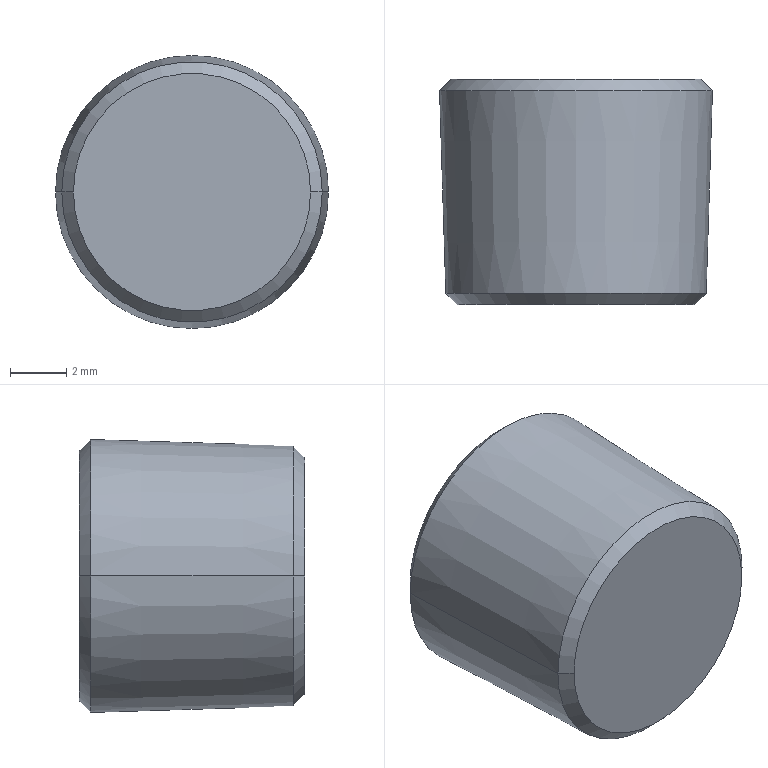Part | Creo | 1 solid | 15 faces | box 9.703 x 8 x 9.703 mm | volume 495.23 mm3 | plane 9 | cone 6
STEP:
#1=CARTESIAN_POINT('',(-108.784,-72.706,-5.5));
#2=VERTEX_POINT('',#1);
#3=CARTESIAN_POINT('',(-117.216,-72.706,-5.5));
#4=VERTEX_POINT('',#3);
#5=CARTESIAN_POINT('',(-113.,-72.706,-5.5));
#6=DIRECTION('',(0.,-1.,0.));
#7=DIRECTION('',(1.,0.,0.));
#8=AXIS2_PLACEMENT_3D('',#5,#6,#7);
#9=CIRCLE('',#8,4.216);
#10=EDGE_CURVE('',#2,#4,#9,.T.);
#11=ORIENTED_EDGE('',*,*,#10,.F.);
#12=CARTESIAN_POINT('',(-113.,-72.706,-5.5));
#13=DIRECTION('',(0.,-1.,0.));
#14=DIRECTION('',(-1.,0.,0.));
#15=AXIS2_PLACEMENT_3D('',#12,#13,#14);
#16=CIRCLE('',#15,4.216);
#17=EDGE_CURVE('',#4,#2,#16,.T.);
#18=ORIENTED_EDGE('',*,*,#17,.F.);
#19=EDGE_LOOP('',(#11,#18));
#20=FACE_OUTER_BOUND('',#19,.F.);
#21=CARTESIAN_POINT('',(-117.616,-72.706,-5.5));
#22=DIRECTION('',(0.,-1.,0.));
#23=DIRECTION('',(1.,0.,0.));
#24=AXIS2_PLACEMENT_3D('',#21,#22,#23);
#25=PLANE('',#24);
#26=ADVANCED_FACE('',(#20),#25,.T.);
#27=ORIENTED_EDGE('',*,*,#10,.T.);
#28=CARTESIAN_POINT('',(-117.628,-72.306,-5.5));
#29=VERTEX_POINT('',#28);
#30=CARTESIAN_POINT('',(-117.216,-72.706,-5.5));
#31=DIRECTION('',(-0.718,0.6961,0.));
#32=VECTOR('',#31,0.5744);
#33=LINE('',#30,#32);
#34=EDGE_CURVE('',#4,#29,#33,.T.);
#35=ORIENTED_EDGE('',*,*,#34,.T.);
#36=CARTESIAN_POINT('',(-108.372,-72.306,-5.5));
#37=VERTEX_POINT('',#36);
#38=CARTESIAN_POINT('',(-113.,-72.306,-5.5));
#39=DIRECTION('',(0.,-1.,0.));
#40=DIRECTION('',(1.,0.,0.));
#41=AXIS2_PLACEMENT_3D('',#38,#39,#40);
#42=CIRCLE('',#41,4.628);
#43=EDGE_CURVE('',#37,#29,#42,.T.);
#44=ORIENTED_EDGE('',*,*,#43,.F.);
#45=CARTESIAN_POINT('',(-108.784,-72.706,-5.5));
#46=DIRECTION('',(0.718,0.6961,0.));
#47=VECTOR('',#46,0.5744);
#48=LINE('',#45,#47);
#49=EDGE_CURVE('',#2,#37,#48,.T.);
#50=ORIENTED_EDGE('',*,*,#49,.F.);
#51=EDGE_LOOP('',(#27,#35,#44,#50));
#52=FACE_OUTER_BOUND('',#51,.F.);
#53=CARTESIAN_POINT('',(-113.,-72.506,-5.5));
#54=DIRECTION('',(0.,1.,0.));
#55=DIRECTION('',(-1.,0.,0.));
#56=AXIS2_PLACEMENT_3D('',#53,#54,#55);
#57=CONICAL_SURFACE('',#56,4.422,45.888);
#58=ADVANCED_FACE('',(#52),#57,.T.);
#59=ORIENTED_EDGE('',*,*,#17,.T.);
#60=ORIENTED_EDGE('',*,*,#49,.T.);
#61=CARTESIAN_POINT('',(-113.,-72.306,-5.5));
#62=DIRECTION('',(0.,-1.,0.));
#63=DIRECTION('',(-1.,0.,0.));
#64=AXIS2_PLACEMENT_3D('',#61,#62,#63);
#65=CIRCLE('',#64,4.628);
#66=EDGE_CURVE('',#29,#37,#65,.T.);
#67=ORIENTED_EDGE('',*,*,#66,.F.);
#68=ORIENTED_EDGE('',*,*,#34,.F.);
#69=EDGE_LOOP('',(#59,#60,#67,#68));
#70=FACE_OUTER_BOUND('',#69,.F.);
#71=CARTESIAN_POINT('',(-113.,-72.506,-5.5));
#72=DIRECTION('',(0.,1.,0.));
#73=DIRECTION('',(-1.,0.,0.));
#74=AXIS2_PLACEMENT_3D('',#71,#72,#73);
#75=CONICAL_SURFACE('',#74,4.422,45.888);
#76=ADVANCED_FACE('',(#70),#75,.T.);
#77=ORIENTED_EDGE('',*,*,#66,.T.);
#78=CARTESIAN_POINT('',(-108.148,-65.106,-5.5));
#79=VERTEX_POINT('',#78);
#80=CARTESIAN_POINT('',(-108.372,-72.306,-5.5));
#81=DIRECTION('',(0.03097,0.9995,0.));
#82=VECTOR('',#81,7.204);
#83=LINE('',#80,#82);
#84=EDGE_CURVE('',#37,#79,#83,.T.);
#85=ORIENTED_EDGE('',*,*,#84,.T.);
#86=CARTESIAN_POINT('',(-117.852,-65.106,-5.5));
#87=VERTEX_POINT('',#86);
#88=CARTESIAN_POINT('',(-113.,-65.106,-5.5));
#89=DIRECTION('',(0.,1.,0.));
#90=DIRECTION('',(1.,0.,0.));
#91=AXIS2_PLACEMENT_3D('',#88,#89,#90);
#92=CIRCLE('',#91,4.852);
#93=EDGE_CURVE('',#79,#87,#92,.T.);
#94=ORIENTED_EDGE('',*,*,#93,.T.);
#95=CARTESIAN_POINT('',(-117.628,-72.306,-5.5));
#96=DIRECTION('',(-0.03097,0.9995,0.));
#97=VECTOR('',#96,7.204);
#98=LINE('',#95,#97);
#99=EDGE_CURVE('',#29,#87,#98,.T.);
#100=ORIENTED_EDGE('',*,*,#99,.F.);
#101=EDGE_LOOP('',(#77,#85,#94,#100));
#102=FACE_OUTER_BOUND('',#101,.F.);
#103=CARTESIAN_POINT('',(-113.,-68.706,-5.5));
#104=DIRECTION('',(0.,1.,0.));
#105=DIRECTION('',(-1.,0.,0.));
#106=AXIS2_PLACEMENT_3D('',#103,#104,#105);
#107=CONICAL_SURFACE('',#106,4.74,1.775);
#108=ADVANCED_FACE('',(#102),#107,.T.);
#109=ORIENTED_EDGE('',*,*,#43,.T.);
#110=ORIENTED_EDGE('',*,*,#99,.T.);
#111=CARTESIAN_POINT('',(-113.,-65.106,-5.5));
#112=DIRECTION('',(0.,1.,0.));
#113=DIRECTION('',(-1.,0.,0.));
#114=AXIS2_PLACEMENT_3D('',#111,#112,#113);
#115=CIRCLE('',#114,4.852);
#116=EDGE_CURVE('',#87,#79,#115,.T.);
#117=ORIENTED_EDGE('',*,*,#116,.T.);
#118=ORIENTED_EDGE('',*,*,#84,.F.);
#119=EDGE_LOOP('',(#109,#110,#117,#118));
#120=FACE_OUTER_BOUND('',#119,.F.);
#121=CARTESIAN_POINT('',(-113.,-68.706,-5.5));
#122=DIRECTION('',(0.,1.,0.));
#123=DIRECTION('',(-1.,0.,0.));
#124=AXIS2_PLACEMENT_3D('',#121,#122,#123);
#125=CONICAL_SURFACE('',#124,4.74,1.775);
#126=ADVANCED_FACE('',(#120),#125,.T.);
#127=ORIENTED_EDGE('',*,*,#116,.F.);
#128=CARTESIAN_POINT('',(-117.464,-64.706,-5.5));
#129=VERTEX_POINT('',#128);
#130=CARTESIAN_POINT('',(-117.464,-64.706,-5.5));
#131=DIRECTION('',(-0.6961,-0.718,0.));
#132=VECTOR('',#131,0.5569);
#133=LINE('',#130,#132);
#134=EDGE_CURVE('',#129,#87,#133,.T.);
#135=ORIENTED_EDGE('',*,*,#134,.F.);
#136=CARTESIAN_POINT('',(-108.536,-64.706,-5.5));
#137=VERTEX_POINT('',#136);
#138=CARTESIAN_POINT('',(-113.,-64.706,-5.5));
#139=DIRECTION('',(0.,1.,0.));
#140=DIRECTION('',(-1.,0.,0.));
#141=AXIS2_PLACEMENT_3D('',#138,#139,#140);
#142=CIRCLE('',#141,4.464);
#143=EDGE_CURVE('',#129,#137,#142,.T.);
#144=ORIENTED_EDGE('',*,*,#143,.T.);
#145=CARTESIAN_POINT('',(-108.536,-64.706,-5.5));
#146=DIRECTION('',(0.6961,-0.718,0.));
#147=VECTOR('',#146,0.5569);
#148=LINE('',#145,#147);
#149=EDGE_CURVE('',#137,#79,#148,.T.);
#150=ORIENTED_EDGE('',*,*,#149,.T.);
#151=EDGE_LOOP('',(#127,#135,#144,#150));
#152=FACE_OUTER_BOUND('',#151,.F.);
#153=CARTESIAN_POINT('',(-113.,-64.906,-5.5));
#154=DIRECTION('',(0.,-1.,0.));
#155=DIRECTION('',(1.,0.,0.));
#156=AXIS2_PLACEMENT_3D('',#153,#154,#155);
#157=CONICAL_SURFACE('',#156,4.658,44.112);
#158=ADVANCED_FACE('',(#152),#157,.T.);
#159=ORIENTED_EDGE('',*,*,#93,.F.);
#160=ORIENTED_EDGE('',*,*,#149,.F.);
#161=CARTESIAN_POINT('',(-113.,-64.706,-5.5));
#162=DIRECTION('',(0.,1.,0.));
#163=DIRECTION('',(1.,0.,0.));
#164=AXIS2_PLACEMENT_3D('',#161,#162,#163);
#165=CIRCLE('',#164,4.464);
#166=EDGE_CURVE('',#137,#129,#165,.T.);
#167=ORIENTED_EDGE('',*,*,#166,.T.);
#168=ORIENTED_EDGE('',*,*,#134,.T.);
#169=EDGE_LOOP('',(#159,#160,#167,#168));
#170=FACE_OUTER_BOUND('',#169,.F.);
#171=CARTESIAN_POINT('',(-113.,-64.906,-5.5));
#172=DIRECTION('',(0.,-1.,0.));
#173=DIRECTION('',(1.,0.,0.));
#174=AXIS2_PLACEMENT_3D('',#171,#172,#173);
#175=CONICAL_SURFACE('',#174,4.658,44.112);
#176=ADVANCED_FACE('',(#170),#175,.T.);
#177=ORIENTED_EDGE('',*,*,#143,.F.);
#178=ORIENTED_EDGE('',*,*,#166,.F.);
#179=EDGE_LOOP('',(#177,#178));
#180=FACE_OUTER_BOUND('',#179,.F.);
#181=CARTESIAN_POINT('',(-111.75,-64.706,-7.665));
#182=VERTEX_POINT('',#181);
#183=CARTESIAN_POINT('',(-110.5,-64.706,-5.5));
#184=VERTEX_POINT('',#183);
#185=CARTESIAN_POINT('',(-111.75,-64.706,-7.665));
#186=DIRECTION('',(0.5,0.,0.866));
#187=VECTOR('',#186,2.5);
#188=LINE('',#185,#187);
#189=EDGE_CURVE('',#182,#184,#188,.T.);
#190=ORIENTED_EDGE('',*,*,#189,.F.);
#191=CARTESIAN_POINT('',(-114.25,-64.706,-7.665));
#192=VERTEX_POINT('',#191);
#193=CARTESIAN_POINT('',(-114.25,-64.706,-7.665));
#194=DIRECTION('',(1.,0.,0.));
#195=VECTOR('',#194,2.5);
#196=LINE('',#193,#195);
#197=EDGE_CURVE('',#192,#182,#196,.T.);
#198=ORIENTED_EDGE('',*,*,#197,.F.);
#199=CARTESIAN_POINT('',(-115.5,-64.706,-5.5));
#200=VERTEX_POINT('',#199);
#201=CARTESIAN_POINT('',(-115.5,-64.706,-5.5));
#202=DIRECTION('',(0.5,0.,-0.866));
#203=VECTOR('',#202,2.5);
#204=LINE('',#201,#203);
#205=EDGE_CURVE('',#200,#192,#204,.T.);
#206=ORIENTED_EDGE('',*,*,#205,.F.);
#207=CARTESIAN_POINT('',(-114.25,-64.706,-3.335));
#208=VERTEX_POINT('',#207);
#209=CARTESIAN_POINT('',(-114.25,-64.706,-3.335));
#210=DIRECTION('',(-0.5,0.,-0.866));
#211=VECTOR('',#210,2.5);
#212=LINE('',#209,#211);
#213=EDGE_CURVE('',#208,#200,#212,.T.);
#214=ORIENTED_EDGE('',*,*,#213,.F.);
#215=CARTESIAN_POINT('',(-111.75,-64.706,-3.335));
#216=VERTEX_POINT('',#215);
#217=CARTESIAN_POINT('',(-111.75,-64.706,-3.335));
#218=DIRECTION('',(-1.,0.,0.));
#219=VECTOR('',#218,2.5);
#220=LINE('',#217,#219);
#221=EDGE_CURVE('',#216,#208,#220,.T.);
#222=ORIENTED_EDGE('',*,*,#221,.F.);
#223=CARTESIAN_POINT('',(-110.5,-64.706,-5.5));
#224=DIRECTION('',(-0.5,0.,0.866));
#225=VECTOR('',#224,2.5);
#226=LINE('',#223,#225);
#227=EDGE_CURVE('',#184,#216,#226,.T.);
#228=ORIENTED_EDGE('',*,*,#227,.F.);
#229=EDGE_LOOP('',(#190,#198,#206,#214,#222,#228));
#230=FACE_BOUND('',#229,.F.);
#231=CARTESIAN_POINT('',(-113.,-64.706,-5.5));
#232=DIRECTION('',(0.,1.,0.));
#233=DIRECTION('',(-1.,0.,0.));
#234=AXIS2_PLACEMENT_3D('',#231,#232,#233);
#235=PLANE('',#234);
#236=ADVANCED_FACE('',(#180,#230),#235,.T.);
#237=ORIENTED_EDGE('',*,*,#189,.T.);
#238=CARTESIAN_POINT('',(-110.5,-68.706,-5.5));
#239=VERTEX_POINT('',#238);
#240=CARTESIAN_POINT('',(-110.5,-68.706,-5.5));
#241=DIRECTION('',(0.,1.,0.));
#242=VECTOR('',#241,4.);
#243=LINE('',#240,#242);
#244=EDGE_CURVE('',#239,#184,#243,.T.);
#245=ORIENTED_EDGE('',*,*,#244,.F.);
#246=CARTESIAN_POINT('',(-111.75,-68.706,-7.665));
#247=VERTEX_POINT('',#246);
#248=CARTESIAN_POINT('',(-110.5,-68.706,-5.5));
#249=DIRECTION('',(-0.5,0.,-0.866));
#250=VECTOR('',#249,2.5);
#251=LINE('',#248,#250);
#252=EDGE_CURVE('',#239,#247,#251,.T.);
#253=ORIENTED_EDGE('',*,*,#252,.T.);
#254=CARTESIAN_POINT('',(-111.75,-68.706,-7.665));
#255=DIRECTION('',(0.,1.,0.));
#256=VECTOR('',#255,4.);
#257=LINE('',#254,#256);
#258=EDGE_CURVE('',#247,#182,#257,.T.);
#259=ORIENTED_EDGE('',*,*,#258,.T.);
#260=EDGE_LOOP('',(#237,#245,#253,#259));
#261=FACE_OUTER_BOUND('',#260,.F.);
#262=CARTESIAN_POINT('',(-110.5,-68.706,-5.5));
#263=DIRECTION('',(0.866,0.,-0.5));
#264=DIRECTION('',(-0.5,0.,-0.866));
#265=AXIS2_PLACEMENT_3D('',#262,#263,#264);
#266=PLANE('',#265);
#267=ADVANCED_FACE('',(#261),#266,.F.);
#268=ORIENTED_EDGE('',*,*,#227,.T.);
#269=CARTESIAN_POINT('',(-111.75,-68.706,-3.335));
#270=VERTEX_POINT('',#269);
#271=CARTESIAN_POINT('',(-111.75,-68.706,-3.335));
#272=DIRECTION('',(0.,1.,0.));
#273=VECTOR('',#272,4.);
#274=LINE('',#271,#273);
#275=EDGE_CURVE('',#270,#216,#274,.T.);
#276=ORIENTED_EDGE('',*,*,#275,.F.);
#277=CARTESIAN_POINT('',(-111.75,-68.706,-3.335));
#278=DIRECTION('',(0.5,0.,-0.866));
#279=VECTOR('',#278,2.5);
#280=LINE('',#277,#279);
#281=EDGE_CURVE('',#270,#239,#280,.T.);
#282=ORIENTED_EDGE('',*,*,#281,.T.);
#283=ORIENTED_EDGE('',*,*,#244,.T.);
#284=EDGE_LOOP('',(#268,#276,#282,#283));
#285=FACE_OUTER_BOUND('',#284,.F.);
#286=CARTESIAN_POINT('',(-111.75,-68.706,-3.335));
#287=DIRECTION('',(0.866,0.,0.5));
#288=DIRECTION('',(0.5,0.,-0.866));
#289=AXIS2_PLACEMENT_3D('',#286,#287,#288);
#290=PLANE('',#289);
#291=ADVANCED_FACE('',(#285),#290,.F.);
#292=ORIENTED_EDGE('',*,*,#221,.T.);
#293=CARTESIAN_POINT('',(-114.25,-68.706,-3.335));
#294=VERTEX_POINT('',#293);
#295=CARTESIAN_POINT('',(-114.25,-68.706,-3.335));
#296=DIRECTION('',(0.,1.,0.));
#297=VECTOR('',#296,4.);
#298=LINE('',#295,#297);
#299=EDGE_CURVE('',#294,#208,#298,.T.);
#300=ORIENTED_EDGE('',*,*,#299,.F.);
#301=CARTESIAN_POINT('',(-114.25,-68.706,-3.335));
#302=DIRECTION('',(1.,0.,0.));
#303=VECTOR('',#302,2.5);
#304=LINE('',#301,#303);
#305=EDGE_CURVE('',#294,#270,#304,.T.);
#306=ORIENTED_EDGE('',*,*,#305,.T.);
#307=ORIENTED_EDGE('',*,*,#275,.T.);
#308=EDGE_LOOP('',(#292,#300,#306,#307));
#309=FACE_OUTER_BOUND('',#308,.F.);
#310=CARTESIAN_POINT('',(-114.25,-68.706,-3.335));
#311=DIRECTION('',(0.,0.,1.));
#312=DIRECTION('',(1.,0.,0.));
#313=AXIS2_PLACEMENT_3D('',#310,#311,#312);
#314=PLANE('',#313);
#315=ADVANCED_FACE('',(#309),#314,.F.);
#316=ORIENTED_EDGE('',*,*,#213,.T.);
#317=CARTESIAN_POINT('',(-115.5,-68.706,-5.5));
#318=VERTEX_POINT('',#317);
#319=CARTESIAN_POINT('',(-115.5,-68.706,-5.5));
#320=DIRECTION('',(0.,1.,0.));
#321=VECTOR('',#320,4.);
#322=LINE('',#319,#321);
#323=EDGE_CURVE('',#318,#200,#322,.T.);
#324=ORIENTED_EDGE('',*,*,#323,.F.);
#325=CARTESIAN_POINT('',(-115.5,-68.706,-5.5));
#326=DIRECTION('',(0.5,0.,0.866));
#327=VECTOR('',#326,2.5);
#328=LINE('',#325,#327);
#329=EDGE_CURVE('',#318,#294,#328,.T.);
#330=ORIENTED_EDGE('',*,*,#329,.T.);
#331=ORIENTED_EDGE('',*,*,#299,.T.);
#332=EDGE_LOOP('',(#316,#324,#330,#331));
#333=FACE_OUTER_BOUND('',#332,.F.);
#334=CARTESIAN_POINT('',(-115.5,-68.706,-5.5));
#335=DIRECTION('',(-0.866,0.,0.5));
#336=DIRECTION('',(0.5,0.,0.866));
#337=AXIS2_PLACEMENT_3D('',#334,#335,#336);
#338=PLANE('',#337);
#339=ADVANCED_FACE('',(#333),#338,.F.);
#340=ORIENTED_EDGE('',*,*,#205,.T.);
#341=CARTESIAN_POINT('',(-114.25,-68.706,-7.665));
#342=VERTEX_POINT('',#341);
#343=CARTESIAN_POINT('',(-114.25,-68.706,-7.665));
#344=DIRECTION('',(0.,1.,0.));
#345=VECTOR('',#344,4.);
#346=LINE('',#343,#345);
#347=EDGE_CURVE('',#342,#192,#346,.T.);
#348=ORIENTED_EDGE('',*,*,#347,.F.);
#349=CARTESIAN_POINT('',(-114.25,-68.706,-7.665));
#350=DIRECTION('',(-0.5,0.,0.866));
#351=VECTOR('',#350,2.5);
#352=LINE('',#349,#351);
#353=EDGE_CURVE('',#342,#318,#352,.T.);
#354=ORIENTED_EDGE('',*,*,#353,.T.);
#355=ORIENTED_EDGE('',*,*,#323,.T.);
#356=EDGE_LOOP('',(#340,#348,#354,#355));
#357=FACE_OUTER_BOUND('',#356,.F.);
#358=CARTESIAN_POINT('',(-114.25,-68.706,-7.665));
#359=DIRECTION('',(-0.866,0.,-0.5));
#360=DIRECTION('',(-0.5,0.,0.866));
#361=AXIS2_PLACEMENT_3D('',#358,#359,#360);
#362=PLANE('',#361);
#363=ADVANCED_FACE('',(#357),#362,.F.);
#364=ORIENTED_EDGE('',*,*,#197,.T.);
#365=ORIENTED_EDGE('',*,*,#258,.F.);
#366=CARTESIAN_POINT('',(-111.75,-68.706,-7.665));
#367=DIRECTION('',(-1.,0.,0.));
#368=VECTOR('',#367,2.5);
#369=LINE('',#366,#368);
#370=EDGE_CURVE('',#247,#342,#369,.T.);
#371=ORIENTED_EDGE('',*,*,#370,.T.);
#372=ORIENTED_EDGE('',*,*,#347,.T.);
#373=EDGE_LOOP('',(#364,#365,#371,#372));
#374=FACE_OUTER_BOUND('',#373,.F.);
#375=CARTESIAN_POINT('',(-111.75,-68.706,-7.665));
#376=DIRECTION('',(0.,0.,-1.));
#377=DIRECTION('',(0.,-1.,0.));
#378=AXIS2_PLACEMENT_3D('',#375,#376,#377);
#379=PLANE('',#378);
#380=ADVANCED_FACE('',(#374),#379,.F.);
#381=ORIENTED_EDGE('',*,*,#252,.F.);
#382=ORIENTED_EDGE('',*,*,#281,.F.);
#383=ORIENTED_EDGE('',*,*,#305,.F.);
#384=ORIENTED_EDGE('',*,*,#329,.F.);
#385=ORIENTED_EDGE('',*,*,#353,.F.);
#386=ORIENTED_EDGE('',*,*,#370,.F.);
#387=EDGE_LOOP('',(#381,#382,#383,#384,#385,#386));
#388=FACE_OUTER_BOUND('',#387,.F.);
#389=CARTESIAN_POINT('',(-113.,-68.706,-5.5));
#390=DIRECTION('',(0.,1.,0.));
#391=DIRECTION('',(-1.,0.,0.));
#392=AXIS2_PLACEMENT_3D('',#389,#390,#391);
#393=PLANE('',#392);
#394=ADVANCED_FACE('',(#388),#393,.T.);
#395=CLOSED_SHELL('',(#26,#58,#76,#108,#126,#158,#176,#236,#267,#291,#315,#339,#363,#380,#394));
#396=MANIFOLD_SOLID_BREP('',#395);
#397=(LENGTH_UNIT()NAMED_UNIT(*)SI_UNIT(.MILLI.,.METRE.));
#398=UNCERTAINTY_MEASURE_WITH_UNIT(LENGTH_MEASURE(0.001588),#397,'','');
#399=(NAMED_UNIT(*)PLANE_ANGLE_UNIT()SI_UNIT($,.RADIAN.));
#400=PLANE_ANGLE_MEASURE_WITH_UNIT(PLANE_ANGLE_MEASURE(0.01745),#399);
#401=(CONVERSION_BASED_UNIT('DEGREE',#400)NAMED_UNIT(*)PLANE_ANGLE_UNIT());
#402=(NAMED_UNIT(*)SI_UNIT($,.STERADIAN.)SOLID_ANGLE_UNIT());
#403=(GEOMETRIC_REPRESENTATION_CONTEXT(3)GLOBAL_UNCERTAINTY_ASSIGNED_CONTEXT((#398))GLOBAL_UNIT_ASSIGNED_CONTEXT((#397,#401,#402))REPRESENTATION_CONTEXT('',''));
#404=ADVANCED_BREP_SHAPE_REPRESENTATION('',(#396),#403);